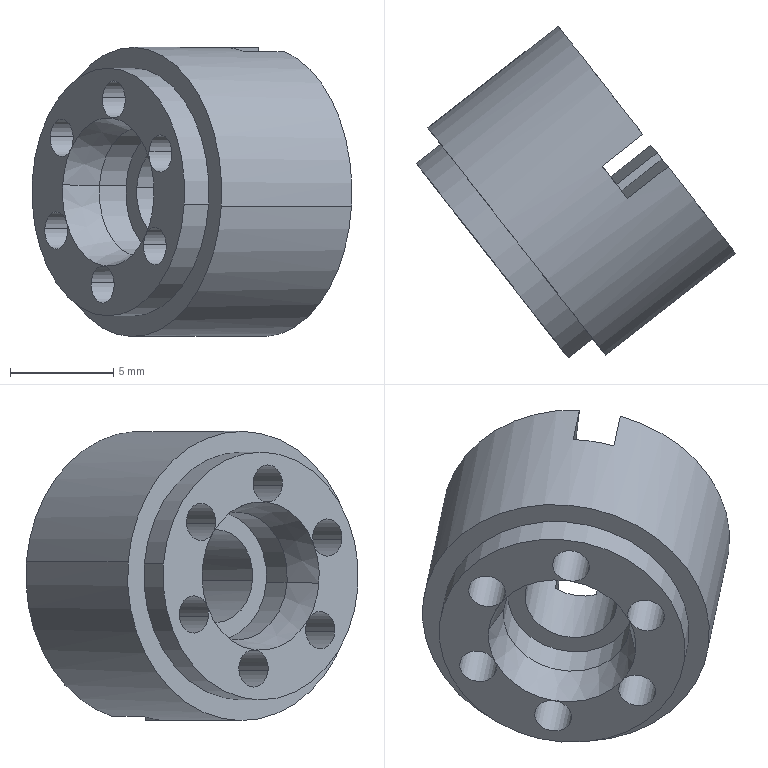Part | SolidWorks | features BaseBody 1 | 1 solid | 33 faces | box 15.49 x 16.093 x 14 mm | volume 1010 mm3 | cylinder 20 | plane 11 | cone 2 | commonest cylinder face diameters 1.8 x12 4.5 x2 6.2 x2 12 x2 14 x2
STEP:
#1=CARTESIAN_POINT('',(2.546,87.739,-118.333));
#2=VERTEX_POINT('',#1);
#3=CARTESIAN_POINT('',(-4.807,97.151,-117.167));
#4=VERTEX_POINT('',#3);
#5=CARTESIAN_POINT('',(-1.131,92.445,-117.75));
#6=DIRECTION('',(-0.788,-0.6157,0.));
#7=DIRECTION('',(0.6128,-0.7843,-0.09712));
#8=AXIS2_PLACEMENT_3D('',#5,#6,#7);
#9=CIRCLE('',#8,6.);
#10=EDGE_CURVE('',#2,#4,#9,.T.);
#11=ORIENTED_EDGE('',*,*,#10,.T.);
#12=CARTESIAN_POINT('',(-5.989,96.227,-117.167));
#13=VERTEX_POINT('',#12);
#14=CARTESIAN_POINT('',(-5.989,96.227,-117.167));
#15=DIRECTION('',(-0.788,-0.6157,0.));
#16=VECTOR('',#15,1000.);
#17=LINE('',#14,#16);
#18=EDGE_CURVE('',#4,#13,#17,.T.);
#19=ORIENTED_EDGE('',*,*,#18,.T.);
#20=CARTESIAN_POINT('',(1.364,86.816,-118.333));
#21=VERTEX_POINT('',#20);
#22=CARTESIAN_POINT('',(-2.313,91.521,-117.75));
#23=DIRECTION('',(-0.788,-0.6157,0.));
#24=DIRECTION('',(0.6128,-0.7843,-0.09712));
#25=AXIS2_PLACEMENT_3D('',#22,#23,#24);
#26=CIRCLE('',#25,6.);
#27=EDGE_CURVE('',#21,#13,#26,.T.);
#28=ORIENTED_EDGE('',*,*,#27,.F.);
#29=CARTESIAN_POINT('',(1.364,86.816,-118.333));
#30=DIRECTION('',(-0.788,-0.6157,0.));
#31=VECTOR('',#30,1000.);
#32=LINE('',#29,#31);
#33=EDGE_CURVE('',#2,#21,#32,.T.);
#34=ORIENTED_EDGE('',*,*,#33,.F.);
#35=EDGE_LOOP('',(#11,#19,#28,#34));
#36=FACE_OUTER_BOUND('',#35,.T.);
#37=CARTESIAN_POINT('',(-2.313,91.521,-117.75));
#38=DIRECTION('',(-0.788,-0.6157,0.));
#39=DIRECTION('',(0.6128,-0.7843,-0.09712));
#40=AXIS2_PLACEMENT_3D('',#37,#38,#39);
#41=CYLINDRICAL_SURFACE('',#40,6.);
#42=ADVANCED_FACE('',(#36),#41,.T.);
#43=CARTESIAN_POINT('',(-2.742,95.102,-117.449));
#44=VERTEX_POINT('',#43);
#45=CARTESIAN_POINT('',(1.057,90.239,-118.051));
#46=VERTEX_POINT('',#45);
#47=CARTESIAN_POINT('',(-0.8423,92.67,-117.75));
#48=DIRECTION('',(-0.788,-0.6157,0.));
#49=DIRECTION('',(0.6128,-0.7843,-0.09712));
#50=AXIS2_PLACEMENT_3D('',#47,#48,#49);
#51=CIRCLE('',#50,3.1);
#52=EDGE_CURVE('',#44,#46,#51,.T.);
#53=ORIENTED_EDGE('',*,*,#52,.F.);
#54=CARTESIAN_POINT('',(-4.519,94.345,-117.4));
#55=VERTEX_POINT('',#54);
#56=CARTESIAN_POINT('',(-2.742,95.102,-117.449));
#57=DIRECTION('',(-0.9198,-0.3917,0.02514));
#58=VECTOR('',#57,1000.);
#59=LINE('',#56,#58);
#60=EDGE_CURVE('',#44,#55,#59,.T.);
#61=ORIENTED_EDGE('',*,*,#60,.T.);
#62=CARTESIAN_POINT('',(-4.331,94.104,-119.239));
#63=VERTEX_POINT('',#62);
#64=CARTESIAN_POINT('',(-2.313,91.521,-117.75));
#65=DIRECTION('',(-0.788,-0.6157,0.));
#66=DIRECTION('',(0.6128,-0.7843,-0.09712));
#67=AXIS2_PLACEMENT_3D('',#64,#65,#66);
#68=CIRCLE('',#67,3.6);
#69=EDGE_CURVE('',#55,#63,#68,.T.);
#70=ORIENTED_EDGE('',*,*,#69,.T.);
#71=CARTESIAN_POINT('',(-2.528,91.797,-121.333));
#72=VERTEX_POINT('',#71);
#73=CARTESIAN_POINT('',(-2.313,91.521,-117.75));
#74=DIRECTION('',(-0.788,-0.6157,0.));
#75=DIRECTION('',(0.6128,-0.7843,-0.09712));
#76=AXIS2_PLACEMENT_3D('',#73,#74,#75);
#77=CIRCLE('',#76,3.6);
#78=EDGE_CURVE('',#63,#72,#77,.T.);
#79=ORIENTED_EDGE('',*,*,#78,.T.);
#80=CARTESIAN_POINT('',(-0.51,89.214,-119.844));
#81=VERTEX_POINT('',#80);
#82=CARTESIAN_POINT('',(-2.313,91.521,-117.75));
#83=DIRECTION('',(-0.788,-0.6157,0.));
#84=DIRECTION('',(0.6128,-0.7843,-0.09712));
#85=AXIS2_PLACEMENT_3D('',#82,#83,#84);
#86=CIRCLE('',#85,3.6);
#87=EDGE_CURVE('',#72,#81,#86,.T.);
#88=ORIENTED_EDGE('',*,*,#87,.T.);
#89=CARTESIAN_POINT('',(-0.1068,88.698,-118.1));
#90=VERTEX_POINT('',#89);
#91=CARTESIAN_POINT('',(-2.313,91.521,-117.75));
#92=DIRECTION('',(-0.788,-0.6157,0.));
#93=DIRECTION('',(0.6128,-0.7843,-0.09712));
#94=AXIS2_PLACEMENT_3D('',#91,#92,#93);
#95=CIRCLE('',#94,3.6);
#96=EDGE_CURVE('',#81,#90,#95,.T.);
#97=ORIENTED_EDGE('',*,*,#96,.T.);
#98=CARTESIAN_POINT('',(1.057,90.239,-118.051));
#99=DIRECTION('',(-0.6026,-0.7977,-0.02514));
#100=VECTOR('',#99,1000.);
#101=LINE('',#98,#100);
#102=EDGE_CURVE('',#46,#90,#101,.T.);
#103=ORIENTED_EDGE('',*,*,#102,.F.);
#104=EDGE_LOOP('',(#53,#61,#70,#79,#88,#97,#103));
#105=FACE_OUTER_BOUND('',#104,.T.);
#106=CARTESIAN_POINT('',(-0.8423,92.67,-117.75));
#107=DIRECTION('',(-0.788,-0.6157,0.));
#108=DIRECTION('',(0.6128,-0.7843,-0.09712));
#109=AXIS2_PLACEMENT_3D('',#106,#107,#108);
#110=CONICAL_SURFACE('',#109,3.1,0.2618);
#111=ADVANCED_FACE('',(#105),#110,.F.);
#112=CARTESIAN_POINT('',(-1.454,96.108,-117.449));
#113=VERTEX_POINT('',#112);
#114=CARTESIAN_POINT('',(2.345,91.245,-118.051));
#115=VERTEX_POINT('',#114);
#116=CARTESIAN_POINT('',(0.4453,93.676,-117.75));
#117=DIRECTION('',(-0.788,-0.6157,0.));
#118=DIRECTION('',(0.6128,-0.7843,-0.09712));
#119=AXIS2_PLACEMENT_3D('',#116,#117,#118);
#120=CIRCLE('',#119,3.1);
#121=EDGE_CURVE('',#113,#115,#120,.T.);
#122=ORIENTED_EDGE('',*,*,#121,.F.);
#123=CARTESIAN_POINT('',(-4.212,93.953,-117.449));
#124=DIRECTION('',(-0.788,-0.6157,0.));
#125=VECTOR('',#124,1000.);
#126=LINE('',#123,#125);
#127=EDGE_CURVE('',#113,#44,#126,.T.);
#128=ORIENTED_EDGE('',*,*,#127,.T.);
#129=ORIENTED_EDGE('',*,*,#52,.T.);
#130=CARTESIAN_POINT('',(-0.4132,89.09,-118.051));
#131=DIRECTION('',(-0.788,-0.6157,0.));
#132=VECTOR('',#131,1000.);
#133=LINE('',#130,#132);
#134=EDGE_CURVE('',#115,#46,#133,.T.);
#135=ORIENTED_EDGE('',*,*,#134,.F.);
#136=EDGE_LOOP('',(#122,#128,#129,#135));
#137=FACE_OUTER_BOUND('',#136,.T.);
#138=CARTESIAN_POINT('',(-2.313,91.521,-117.75));
#139=DIRECTION('',(-0.788,-0.6157,0.));
#140=DIRECTION('',(0.6128,-0.7843,-0.09712));
#141=AXIS2_PLACEMENT_3D('',#138,#139,#140);
#142=CYLINDRICAL_SURFACE('',#141,3.1);
#143=ADVANCED_FACE('',(#137),#142,.F.);
#144=CARTESIAN_POINT('',(3.795,99.135,-117.531));
#145=VERTEX_POINT('',#144);
#146=CARTESIAN_POINT('',(4.44,98.309,-119.659));
#147=VERTEX_POINT('',#146);
#148=CARTESIAN_POINT('',(5.173,97.37,-117.75));
#149=DIRECTION('',(-0.788,-0.6157,0.));
#150=DIRECTION('',(0.6128,-0.7843,-0.09712));
#151=AXIS2_PLACEMENT_3D('',#148,#149,#150);
#152=CIRCLE('',#151,2.25);
#153=EDGE_CURVE('',#145,#147,#152,.T.);
#154=ORIENTED_EDGE('',*,*,#153,.F.);
#155=CARTESIAN_POINT('',(-0.9334,95.441,-117.531));
#156=VERTEX_POINT('',#155);
#157=CARTESIAN_POINT('',(-3.691,93.286,-117.531));
#158=DIRECTION('',(-0.788,-0.6157,0.));
#159=VECTOR('',#158,1000.);
#160=LINE('',#157,#159);
#161=EDGE_CURVE('',#145,#156,#160,.T.);
#162=ORIENTED_EDGE('',*,*,#161,.T.);
#163=CARTESIAN_POINT('',(1.824,91.912,-117.969));
#164=VERTEX_POINT('',#163);
#165=CARTESIAN_POINT('',(0.4453,93.676,-117.75));
#166=DIRECTION('',(-0.788,-0.6157,0.));
#167=DIRECTION('',(0.6128,-0.7843,-0.09712));
#168=AXIS2_PLACEMENT_3D('',#165,#166,#167);
#169=CIRCLE('',#168,2.25);
#170=EDGE_CURVE('',#156,#164,#169,.T.);
#171=ORIENTED_EDGE('',*,*,#170,.T.);
#172=CARTESIAN_POINT('',(6.552,95.606,-117.969));
#173=VERTEX_POINT('',#172);
#174=CARTESIAN_POINT('',(-0.934,89.757,-117.969));
#175=DIRECTION('',(-0.788,-0.6157,0.));
#176=VECTOR('',#175,1000.);
#177=LINE('',#174,#176);
#178=EDGE_CURVE('',#173,#164,#177,.T.);
#179=ORIENTED_EDGE('',*,*,#178,.F.);
#180=CARTESIAN_POINT('',(5.666,96.74,-119.853));
#181=VERTEX_POINT('',#180);
#182=CARTESIAN_POINT('',(5.173,97.37,-117.75));
#183=DIRECTION('',(-0.788,-0.6157,0.));
#184=DIRECTION('',(0.6128,-0.7843,-0.09712));
#185=AXIS2_PLACEMENT_3D('',#182,#183,#184);
#186=CIRCLE('',#185,2.25);
#187=EDGE_CURVE('',#181,#173,#186,.T.);
#188=ORIENTED_EDGE('',*,*,#187,.F.);
#189=CARTESIAN_POINT('',(3.696,95.201,-119.853));
#190=VERTEX_POINT('',#189);
#191=CARTESIAN_POINT('',(-1.82,90.891,-119.853));
#192=DIRECTION('',(0.788,0.6157,0.));
#193=VECTOR('',#192,1000.);
#194=LINE('',#191,#193);
#195=EDGE_CURVE('',#190,#181,#194,.T.);
#196=ORIENTED_EDGE('',*,*,#195,.F.);
#197=CARTESIAN_POINT('',(2.47,96.77,-119.659));
#198=VERTEX_POINT('',#197);
#199=CARTESIAN_POINT('',(3.203,95.831,-117.75));
#200=DIRECTION('',(0.788,0.6157,0.));
#201=DIRECTION('',(-0.6128,0.7843,0.09712));
#202=AXIS2_PLACEMENT_3D('',#199,#200,#201);
#203=CIRCLE('',#202,2.25);
#204=EDGE_CURVE('',#190,#198,#203,.T.);
#205=ORIENTED_EDGE('',*,*,#204,.T.);
#206=CARTESIAN_POINT('',(-3.046,92.46,-119.659));
#207=DIRECTION('',(-0.788,-0.6157,0.));
#208=VECTOR('',#207,1000.);
#209=LINE('',#206,#208);
#210=EDGE_CURVE('',#147,#198,#209,.T.);
#211=ORIENTED_EDGE('',*,*,#210,.F.);
#212=EDGE_LOOP('',(#154,#162,#171,#179,#188,#196,#205,#211));
#213=FACE_OUTER_BOUND('',#212,.T.);
#214=CARTESIAN_POINT('',(-2.313,91.521,-117.75));
#215=DIRECTION('',(-0.788,-0.6157,0.));
#216=DIRECTION('',(0.6128,-0.7843,-0.09712));
#217=AXIS2_PLACEMENT_3D('',#214,#215,#216);
#218=CYLINDRICAL_SURFACE('',#217,2.25);
#219=ADVANCED_FACE('',(#213),#218,.F.);
#220=CARTESIAN_POINT('',(4.975,97.624,-110.757));
#221=VERTEX_POINT('',#220);
#222=CARTESIAN_POINT('',(0.8841,102.86,-117.07));
#223=VERTEX_POINT('',#222);
#224=CARTESIAN_POINT('',(5.173,97.37,-117.75));
#225=DIRECTION('',(-0.788,-0.6157,0.));
#226=DIRECTION('',(0.6128,-0.7843,-0.09712));
#227=AXIS2_PLACEMENT_3D('',#224,#225,#226);
#228=CIRCLE('',#227,7.);
#229=EDGE_CURVE('',#221,#223,#228,.T.);
#230=ORIENTED_EDGE('',*,*,#229,.T.);
#231=CARTESIAN_POINT('',(-5.42,97.935,-117.07));
#232=VERTEX_POINT('',#231);
#233=CARTESIAN_POINT('',(-6.602,97.011,-117.07));
#234=DIRECTION('',(-0.788,-0.6157,0.));
#235=VECTOR('',#234,1000.);
#236=LINE('',#233,#235);
#237=EDGE_CURVE('',#223,#232,#236,.T.);
#238=ORIENTED_EDGE('',*,*,#237,.T.);
#239=CARTESIAN_POINT('',(3.159,86.955,-118.43));
#240=VERTEX_POINT('',#239);
#241=CARTESIAN_POINT('',(-1.131,92.445,-117.75));
#242=DIRECTION('',(-0.788,-0.6157,0.));
#243=DIRECTION('',(0.6128,-0.7843,-0.09712));
#244=AXIS2_PLACEMENT_3D('',#241,#242,#243);
#245=CIRCLE('',#244,7.);
#246=EDGE_CURVE('',#240,#232,#245,.T.);
#247=ORIENTED_EDGE('',*,*,#246,.F.);
#248=CARTESIAN_POINT('',(9.463,91.88,-118.43));
#249=VERTEX_POINT('',#248);
#250=CARTESIAN_POINT('',(1.977,86.031,-118.43));
#251=DIRECTION('',(-0.788,-0.6157,0.));
#252=VECTOR('',#251,1000.);
#253=LINE('',#250,#252);
#254=EDGE_CURVE('',#249,#240,#253,.T.);
#255=ORIENTED_EDGE('',*,*,#254,.F.);
#256=CARTESIAN_POINT('',(6.2,96.056,-110.952));
#257=VERTEX_POINT('',#256);
#258=CARTESIAN_POINT('',(5.173,97.37,-117.75));
#259=DIRECTION('',(-0.788,-0.6157,0.));
#260=DIRECTION('',(0.6128,-0.7843,-0.09712));
#261=AXIS2_PLACEMENT_3D('',#258,#259,#260);
#262=CIRCLE('',#261,7.);
#263=EDGE_CURVE('',#249,#257,#262,.T.);
#264=ORIENTED_EDGE('',*,*,#263,.T.);
#265=CARTESIAN_POINT('',(4.23,94.517,-110.952));
#266=VERTEX_POINT('',#265);
#267=CARTESIAN_POINT('',(4.23,94.517,-110.952));
#268=DIRECTION('',(0.788,0.6157,0.));
#269=VECTOR('',#268,1000.);
#270=LINE('',#267,#269);
#271=EDGE_CURVE('',#266,#257,#270,.T.);
#272=ORIENTED_EDGE('',*,*,#271,.F.);
#273=CARTESIAN_POINT('',(3.005,96.085,-110.757));
#274=VERTEX_POINT('',#273);
#275=CARTESIAN_POINT('',(3.203,95.831,-117.75));
#276=DIRECTION('',(0.788,0.6157,0.));
#277=DIRECTION('',(-0.6128,0.7843,0.09712));
#278=AXIS2_PLACEMENT_3D('',#275,#276,#277);
#279=CIRCLE('',#278,7.);
#280=EDGE_CURVE('',#274,#266,#279,.T.);
#281=ORIENTED_EDGE('',*,*,#280,.F.);
#282=CARTESIAN_POINT('',(3.005,96.085,-110.757));
#283=DIRECTION('',(0.788,0.6157,0.));
#284=VECTOR('',#283,1000.);
#285=LINE('',#282,#284);
#286=EDGE_CURVE('',#274,#221,#285,.T.);
#287=ORIENTED_EDGE('',*,*,#286,.T.);
#288=EDGE_LOOP('',(#230,#238,#247,#255,#264,#272,#281,#287));
#289=FACE_OUTER_BOUND('',#288,.T.);
#290=CARTESIAN_POINT('',(-2.313,91.521,-117.75));
#291=DIRECTION('',(-0.788,-0.6157,0.));
#292=DIRECTION('',(0.6128,-0.7843,-0.09712));
#293=AXIS2_PLACEMENT_3D('',#290,#291,#292);
#294=CYLINDRICAL_SURFACE('',#293,7.);
#295=ADVANCED_FACE('',(#289),#294,.T.);
#296=CARTESIAN_POINT('',(-1.492,90.471,-113.359));
#297=VERTEX_POINT('',#296);
#298=CARTESIAN_POINT('',(-2.097,91.246,-114.167));
#299=VERTEX_POINT('',#298);
#300=CARTESIAN_POINT('',(-2.044,91.177,-113.271));
#301=DIRECTION('',(0.788,0.6157,0.));
#302=DIRECTION('',(-0.6128,0.7843,0.09712));
#303=AXIS2_PLACEMENT_3D('',#300,#301,#302);
#304=CIRCLE('',#303,0.9);
#305=EDGE_CURVE('',#297,#299,#304,.T.);
#306=ORIENTED_EDGE('',*,*,#305,.F.);
#307=CARTESIAN_POINT('',(4.024,94.781,-113.359));
#308=VERTEX_POINT('',#307);
#309=CARTESIAN_POINT('',(-1.492,90.471,-113.359));
#310=DIRECTION('',(0.788,0.6157,0.));
#311=VECTOR('',#310,1000.);
#312=LINE('',#309,#311);
#313=EDGE_CURVE('',#297,#308,#312,.T.);
#314=ORIENTED_EDGE('',*,*,#313,.T.);
#315=CARTESIAN_POINT('',(2.921,96.192,-113.184));
#316=VERTEX_POINT('',#315);
#317=CARTESIAN_POINT('',(3.472,95.487,-113.271));
#318=DIRECTION('',(0.788,0.6157,0.));
#319=DIRECTION('',(-0.6128,0.7843,0.09712));
#320=AXIS2_PLACEMENT_3D('',#317,#318,#319);
#321=CIRCLE('',#320,0.9);
#322=EDGE_CURVE('',#308,#316,#321,.T.);
#323=ORIENTED_EDGE('',*,*,#322,.T.);
#324=CARTESIAN_POINT('',(-2.595,91.883,-113.184));
#325=VERTEX_POINT('',#324);
#326=CARTESIAN_POINT('',(-2.595,91.883,-113.184));
#327=DIRECTION('',(0.788,0.6157,0.));
#328=VECTOR('',#327,1000.);
#329=LINE('',#326,#328);
#330=EDGE_CURVE('',#325,#316,#329,.T.);
#331=ORIENTED_EDGE('',*,*,#330,.F.);
#332=CARTESIAN_POINT('',(-2.044,91.177,-113.271));
#333=DIRECTION('',(0.788,0.6157,0.));
#334=DIRECTION('',(-0.6128,0.7843,0.09712));
#335=AXIS2_PLACEMENT_3D('',#332,#333,#334);
#336=CIRCLE('',#335,0.9);
#337=EDGE_CURVE('',#299,#325,#336,.T.);
#338=ORIENTED_EDGE('',*,*,#337,.F.);
#339=EDGE_LOOP('',(#306,#314,#323,#331,#338));
#340=FACE_OUTER_BOUND('',#339,.T.);
#341=CARTESIAN_POINT('',(-2.044,91.177,-113.271));
#342=DIRECTION('',(0.788,0.6157,0.));
#343=DIRECTION('',(-0.6128,0.7843,0.09712));
#344=AXIS2_PLACEMENT_3D('',#341,#342,#343);
#345=CYLINDRICAL_SURFACE('',#344,0.9);
#346=ADVANCED_FACE('',(#340),#345,.F.);
#347=CARTESIAN_POINT('',(-4.015,93.7,-115.22));
#348=VERTEX_POINT('',#347);
#349=CARTESIAN_POINT('',(-4.115,93.829,-115.656));
#350=VERTEX_POINT('',#349);
#351=CARTESIAN_POINT('',(-4.566,94.406,-115.132));
#352=DIRECTION('',(0.788,0.6157,0.));
#353=DIRECTION('',(-0.6128,0.7843,0.09712));
#354=AXIS2_PLACEMENT_3D('',#351,#352,#353);
#355=CIRCLE('',#354,0.9);
#356=EDGE_CURVE('',#348,#350,#355,.T.);
#357=ORIENTED_EDGE('',*,*,#356,.F.);
#358=CARTESIAN_POINT('',(3.471,99.549,-115.22));
#359=VERTEX_POINT('',#358);
#360=CARTESIAN_POINT('',(-4.015,93.7,-115.22));
#361=DIRECTION('',(0.788,0.6157,0.));
#362=VECTOR('',#361,1000.);
#363=LINE('',#360,#362);
#364=EDGE_CURVE('',#348,#359,#363,.T.);
#365=ORIENTED_EDGE('',*,*,#364,.T.);
#366=CARTESIAN_POINT('',(2.368,100.96,-115.045));
#367=VERTEX_POINT('',#366);
#368=CARTESIAN_POINT('',(2.92,100.254,-115.132));
#369=DIRECTION('',(0.788,0.6157,0.));
#370=DIRECTION('',(-0.6128,0.7843,0.09712));
#371=AXIS2_PLACEMENT_3D('',#368,#369,#370);
#372=CIRCLE('',#371,0.9);
#373=EDGE_CURVE('',#359,#367,#372,.T.);
#374=ORIENTED_EDGE('',*,*,#373,.T.);
#375=CARTESIAN_POINT('',(-5.118,95.112,-115.045));
#376=VERTEX_POINT('',#375);
#377=CARTESIAN_POINT('',(-5.118,95.112,-115.045));
#378=DIRECTION('',(0.788,0.6157,0.));
#379=VECTOR('',#378,1000.);
#380=LINE('',#377,#379);
#381=EDGE_CURVE('',#376,#367,#380,.T.);
#382=ORIENTED_EDGE('',*,*,#381,.F.);
#383=CARTESIAN_POINT('',(-4.566,94.406,-115.132));
#384=DIRECTION('',(0.788,0.6157,0.));
#385=DIRECTION('',(-0.6128,0.7843,0.09712));
#386=AXIS2_PLACEMENT_3D('',#383,#384,#385);
#387=CIRCLE('',#386,0.9);
#388=EDGE_CURVE('',#350,#376,#387,.T.);
#389=ORIENTED_EDGE('',*,*,#388,.F.);
#390=EDGE_LOOP('',(#357,#365,#374,#382,#389));
#391=FACE_OUTER_BOUND('',#390,.T.);
#392=CARTESIAN_POINT('',(-4.566,94.406,-115.132));
#393=DIRECTION('',(0.788,0.6157,0.));
#394=DIRECTION('',(-0.6128,0.7843,0.09712));
#395=AXIS2_PLACEMENT_3D('',#392,#393,#394);
#396=CYLINDRICAL_SURFACE('',#395,0.9);
#397=ADVANCED_FACE('',(#391),#396,.F.);
#398=CARTESIAN_POINT('',(-4.284,94.044,-119.698));
#399=VERTEX_POINT('',#398);
#400=CARTESIAN_POINT('',(-5.387,95.456,-119.523));
#401=VERTEX_POINT('',#400);
#402=CARTESIAN_POINT('',(-4.835,94.75,-119.611));
#403=DIRECTION('',(0.788,0.6157,0.));
#404=DIRECTION('',(-0.6128,0.7843,0.09712));
#405=AXIS2_PLACEMENT_3D('',#402,#403,#404);
#406=CIRCLE('',#405,0.9);
#407=EDGE_CURVE('',#399,#401,#406,.T.);
#408=ORIENTED_EDGE('',*,*,#407,.F.);
#409=CARTESIAN_POINT('',(3.202,99.893,-119.698));
#410=VERTEX_POINT('',#409);
#411=CARTESIAN_POINT('',(-4.284,94.044,-119.698));
#412=DIRECTION('',(0.788,0.6157,0.));
#413=VECTOR('',#412,1000.);
#414=LINE('',#411,#413);
#415=EDGE_CURVE('',#399,#410,#414,.T.);
#416=ORIENTED_EDGE('',*,*,#415,.T.);
#417=CARTESIAN_POINT('',(2.099,101.305,-119.523));
#418=VERTEX_POINT('',#417);
#419=CARTESIAN_POINT('',(2.651,100.599,-119.611));
#420=DIRECTION('',(0.788,0.6157,0.));
#421=DIRECTION('',(-0.6128,0.7843,0.09712));
#422=AXIS2_PLACEMENT_3D('',#419,#420,#421);
#423=CIRCLE('',#422,0.9);
#424=EDGE_CURVE('',#410,#418,#423,.T.);
#425=ORIENTED_EDGE('',*,*,#424,.T.);
#426=CARTESIAN_POINT('',(-5.387,95.456,-119.523));
#427=DIRECTION('',(0.788,0.6157,0.));
#428=VECTOR('',#427,1000.);
#429=LINE('',#426,#428);
#430=EDGE_CURVE('',#401,#418,#429,.T.);
#431=ORIENTED_EDGE('',*,*,#430,.F.);
#432=EDGE_LOOP('',(#408,#416,#425,#431));
#433=FACE_OUTER_BOUND('',#432,.T.);
#434=CARTESIAN_POINT('',(-4.835,94.75,-119.611));
#435=DIRECTION('',(0.788,0.6157,0.));
#436=DIRECTION('',(-0.6128,0.7843,0.09712));
#437=AXIS2_PLACEMENT_3D('',#434,#435,#436);
#438=CYLINDRICAL_SURFACE('',#437,0.9);
#439=ADVANCED_FACE('',(#433),#438,.F.);
#440=CARTESIAN_POINT('',(-2.03,91.16,-122.316));
#441=VERTEX_POINT('',#440);
#442=CARTESIAN_POINT('',(-3.133,92.572,-122.141));
#443=VERTEX_POINT('',#442);
#444=CARTESIAN_POINT('',(-2.582,91.866,-122.229));
#445=DIRECTION('',(0.788,0.6157,0.));
#446=DIRECTION('',(-0.6128,0.7843,0.09712));
#447=AXIS2_PLACEMENT_3D('',#444,#445,#446);
#448=CIRCLE('',#447,0.9);
#449=EDGE_CURVE('',#441,#443,#448,.T.);
#450=ORIENTED_EDGE('',*,*,#449,.F.);
#451=CARTESIAN_POINT('',(3.486,95.47,-122.316));
#452=VERTEX_POINT('',#451);
#453=CARTESIAN_POINT('',(-2.03,91.16,-122.316));
#454=DIRECTION('',(0.788,0.6157,0.));
#455=VECTOR('',#454,1000.);
#456=LINE('',#453,#455);
#457=EDGE_CURVE('',#441,#452,#456,.T.);
#458=ORIENTED_EDGE('',*,*,#457,.T.);
#459=CARTESIAN_POINT('',(2.383,96.881,-122.141));
#460=VERTEX_POINT('',#459);
#461=CARTESIAN_POINT('',(2.934,96.175,-122.229));
#462=DIRECTION('',(0.788,0.6157,0.));
#463=DIRECTION('',(-0.6128,0.7843,0.09712));
#464=AXIS2_PLACEMENT_3D('',#461,#462,#463);
#465=CIRCLE('',#464,0.9);
#466=EDGE_CURVE('',#452,#460,#465,.T.);
#467=ORIENTED_EDGE('',*,*,#466,.T.);
#468=CARTESIAN_POINT('',(-3.133,92.572,-122.141));
#469=DIRECTION('',(0.788,0.6157,0.));
#470=VECTOR('',#469,1000.);
#471=LINE('',#468,#470);
#472=EDGE_CURVE('',#443,#460,#471,.T.);
#473=ORIENTED_EDGE('',*,*,#472,.F.);
#474=EDGE_LOOP('',(#450,#458,#467,#473));
#475=FACE_OUTER_BOUND('',#474,.T.);
#476=CARTESIAN_POINT('',(-2.582,91.866,-122.229));
#477=DIRECTION('',(0.788,0.6157,0.));
#478=DIRECTION('',(-0.6128,0.7843,0.09712));
#479=AXIS2_PLACEMENT_3D('',#476,#477,#478);
#480=CYLINDRICAL_SURFACE('',#479,0.9);
#481=ADVANCED_FACE('',(#475),#480,.F.);
#482=CARTESIAN_POINT('',(0.4922,87.931,-120.455));
#483=VERTEX_POINT('',#482);
#484=CARTESIAN_POINT('',(-0.6108,89.343,-120.28));
#485=VERTEX_POINT('',#484);
#486=CARTESIAN_POINT('',(-0.05931,88.637,-120.368));
#487=DIRECTION('',(0.788,0.6157,0.));
#488=DIRECTION('',(-0.6128,0.7843,0.09712));
#489=AXIS2_PLACEMENT_3D('',#486,#487,#488);
#490=CIRCLE('',#489,0.9);
#491=EDGE_CURVE('',#483,#485,#490,.T.);
#492=ORIENTED_EDGE('',*,*,#491,.F.);
#493=CARTESIAN_POINT('',(7.978,93.78,-120.455));
#494=VERTEX_POINT('',#493);
#495=CARTESIAN_POINT('',(0.4922,87.931,-120.455));
#496=DIRECTION('',(0.788,0.6157,0.));
#497=VECTOR('',#496,1000.);
#498=LINE('',#495,#497);
#499=EDGE_CURVE('',#483,#494,#498,.T.);
#500=ORIENTED_EDGE('',*,*,#499,.T.);
#501=CARTESIAN_POINT('',(6.875,95.192,-120.28));
#502=VERTEX_POINT('',#501);
#503=CARTESIAN_POINT('',(7.427,94.486,-120.368));
#504=DIRECTION('',(0.788,0.6157,0.));
#505=DIRECTION('',(-0.6128,0.7843,0.09712));
#506=AXIS2_PLACEMENT_3D('',#503,#504,#505);
#507=CIRCLE('',#506,0.9);
#508=EDGE_CURVE('',#494,#502,#507,.T.);
#509=ORIENTED_EDGE('',*,*,#508,.T.);
#510=CARTESIAN_POINT('',(-0.6108,89.343,-120.28));
#511=DIRECTION('',(0.788,0.6157,0.));
#512=VECTOR('',#511,1000.);
#513=LINE('',#510,#512);
#514=EDGE_CURVE('',#485,#502,#513,.T.);
#515=ORIENTED_EDGE('',*,*,#514,.F.);
#516=EDGE_LOOP('',(#492,#500,#509,#515));
#517=FACE_OUTER_BOUND('',#516,.T.);
#518=CARTESIAN_POINT('',(-0.05931,88.637,-120.368));
#519=DIRECTION('',(0.788,0.6157,0.));
#520=DIRECTION('',(-0.6128,0.7843,0.09712));
#521=AXIS2_PLACEMENT_3D('',#518,#519,#520);
#522=CYLINDRICAL_SURFACE('',#521,0.9);
#523=ADVANCED_FACE('',(#517),#522,.F.);
#524=CARTESIAN_POINT('',(0.7612,87.587,-115.977));
#525=VERTEX_POINT('',#524);
#526=CARTESIAN_POINT('',(-0.2947,88.938,-116.261));
#527=VERTEX_POINT('',#526);
#528=CARTESIAN_POINT('',(0.2098,88.293,-115.889));
#529=DIRECTION('',(0.788,0.6157,0.));
#530=DIRECTION('',(-0.6128,0.7843,0.09712));
#531=AXIS2_PLACEMENT_3D('',#528,#529,#530);
#532=CIRCLE('',#531,0.9);
#533=EDGE_CURVE('',#525,#527,#532,.T.);
#534=ORIENTED_EDGE('',*,*,#533,.F.);
#535=CARTESIAN_POINT('',(8.247,93.436,-115.977));
#536=VERTEX_POINT('',#535);
#537=CARTESIAN_POINT('',(0.7612,87.587,-115.977));
#538=DIRECTION('',(0.788,0.6157,0.));
#539=VECTOR('',#538,1000.);
#540=LINE('',#537,#539);
#541=EDGE_CURVE('',#525,#536,#540,.T.);
#542=ORIENTED_EDGE('',*,*,#541,.T.);
#543=CARTESIAN_POINT('',(7.144,94.847,-115.802));
#544=VERTEX_POINT('',#543);
#545=CARTESIAN_POINT('',(7.696,94.142,-115.889));
#546=DIRECTION('',(0.788,0.6157,0.));
#547=DIRECTION('',(-0.6128,0.7843,0.09712));
#548=AXIS2_PLACEMENT_3D('',#545,#546,#547);
#549=CIRCLE('',#548,0.9);
#550=EDGE_CURVE('',#536,#544,#549,.T.);
#551=ORIENTED_EDGE('',*,*,#550,.T.);
#552=CARTESIAN_POINT('',(-0.3417,88.999,-115.802));
#553=VERTEX_POINT('',#552);
#554=CARTESIAN_POINT('',(-0.3417,88.999,-115.802));
#555=DIRECTION('',(0.788,0.6157,0.));
#556=VECTOR('',#555,1000.);
#557=LINE('',#554,#556);
#558=EDGE_CURVE('',#553,#544,#557,.T.);
#559=ORIENTED_EDGE('',*,*,#558,.F.);
#560=CARTESIAN_POINT('',(0.2098,88.293,-115.889));
#561=DIRECTION('',(0.788,0.6157,0.));
#562=DIRECTION('',(-0.6128,0.7843,0.09712));
#563=AXIS2_PLACEMENT_3D('',#560,#561,#562);
#564=CIRCLE('',#563,0.9);
#565=EDGE_CURVE('',#527,#553,#564,.T.);
#566=ORIENTED_EDGE('',*,*,#565,.F.);
#567=EDGE_LOOP('',(#534,#542,#551,#559,#566));
#568=FACE_OUTER_BOUND('',#567,.T.);
#569=CARTESIAN_POINT('',(0.2098,88.293,-115.889));
#570=DIRECTION('',(0.788,0.6157,0.));
#571=DIRECTION('',(-0.6128,0.7843,0.09712));
#572=AXIS2_PLACEMENT_3D('',#569,#570,#571);
#573=CYLINDRICAL_SURFACE('',#572,0.9);
#574=ADVANCED_FACE('',(#568),#573,.F.);
#575=ORIENTED_EDGE('',*,*,#541,.F.);
#576=CARTESIAN_POINT('',(0.2098,88.293,-115.889));
#577=DIRECTION('',(0.788,0.6157,0.));
#578=DIRECTION('',(-0.6128,0.7843,0.09712));
#579=AXIS2_PLACEMENT_3D('',#576,#577,#578);
#580=CIRCLE('',#579,0.9);
#581=EDGE_CURVE('',#553,#525,#580,.T.);
#582=ORIENTED_EDGE('',*,*,#581,.F.);
#583=ORIENTED_EDGE('',*,*,#558,.T.);
#584=CARTESIAN_POINT('',(7.696,94.142,-115.889));
#585=DIRECTION('',(0.788,0.6157,0.));
#586=DIRECTION('',(-0.6128,0.7843,0.09712));
#587=AXIS2_PLACEMENT_3D('',#584,#585,#586);
#588=CIRCLE('',#587,0.9);
#589=EDGE_CURVE('',#544,#536,#588,.T.);
#590=ORIENTED_EDGE('',*,*,#589,.T.);
#591=EDGE_LOOP('',(#575,#582,#583,#590));
#592=FACE_OUTER_BOUND('',#591,.T.);
#593=CARTESIAN_POINT('',(0.2098,88.293,-115.889));
#594=DIRECTION('',(0.788,0.6157,0.));
#595=DIRECTION('',(-0.6128,0.7843,0.09712));
#596=AXIS2_PLACEMENT_3D('',#593,#594,#595);
#597=CYLINDRICAL_SURFACE('',#596,0.9);
#598=ADVANCED_FACE('',(#592),#597,.F.);
#599=ORIENTED_EDGE('',*,*,#499,.F.);
#600=CARTESIAN_POINT('',(-0.05931,88.637,-120.368));
#601=DIRECTION('',(0.788,0.6157,0.));
#602=DIRECTION('',(-0.6128,0.7843,0.09712));
#603=AXIS2_PLACEMENT_3D('',#600,#601,#602);
#604=CIRCLE('',#603,0.9);
#605=EDGE_CURVE('',#81,#483,#604,.T.);
#606=ORIENTED_EDGE('',*,*,#605,.F.);
#607=CARTESIAN_POINT('',(-0.05931,88.637,-120.368));
#608=DIRECTION('',(0.788,0.6157,0.));
#609=DIRECTION('',(-0.6128,0.7843,0.09712));
#610=AXIS2_PLACEMENT_3D('',#607,#608,#609);
#611=CIRCLE('',#610,0.9);
#612=EDGE_CURVE('',#485,#81,#611,.T.);
#613=ORIENTED_EDGE('',*,*,#612,.F.);
#614=ORIENTED_EDGE('',*,*,#514,.T.);
#615=CARTESIAN_POINT('',(7.427,94.486,-120.368));
#616=DIRECTION('',(0.788,0.6157,0.));
#617=DIRECTION('',(-0.6128,0.7843,0.09712));
#618=AXIS2_PLACEMENT_3D('',#615,#616,#617);
#619=CIRCLE('',#618,0.9);
#620=EDGE_CURVE('',#502,#494,#619,.T.);
#621=ORIENTED_EDGE('',*,*,#620,.T.);
#622=EDGE_LOOP('',(#599,#606,#613,#614,#621));
#623=FACE_OUTER_BOUND('',#622,.T.);
#624=CARTESIAN_POINT('',(-0.05931,88.637,-120.368));
#625=DIRECTION('',(0.788,0.6157,0.));
#626=DIRECTION('',(-0.6128,0.7843,0.09712));
#627=AXIS2_PLACEMENT_3D('',#624,#625,#626);
#628=CYLINDRICAL_SURFACE('',#627,0.9);
#629=ADVANCED_FACE('',(#623),#628,.F.);
#630=ORIENTED_EDGE('',*,*,#457,.F.);
#631=CARTESIAN_POINT('',(-2.582,91.866,-122.229));
#632=DIRECTION('',(0.788,0.6157,0.));
#633=DIRECTION('',(-0.6128,0.7843,0.09712));
#634=AXIS2_PLACEMENT_3D('',#631,#632,#633);
#635=CIRCLE('',#634,0.9);
#636=EDGE_CURVE('',#72,#441,#635,.T.);
#637=ORIENTED_EDGE('',*,*,#636,.F.);
#638=CARTESIAN_POINT('',(-2.582,91.866,-122.229));
#639=DIRECTION('',(0.788,0.6157,0.));
#640=DIRECTION('',(-0.6128,0.7843,0.09712));
#641=AXIS2_PLACEMENT_3D('',#638,#639,#640);
#642=CIRCLE('',#641,0.9);
#643=EDGE_CURVE('',#443,#72,#642,.T.);
#644=ORIENTED_EDGE('',*,*,#643,.F.);
#645=ORIENTED_EDGE('',*,*,#472,.T.);
#646=CARTESIAN_POINT('',(2.934,96.175,-122.229));
#647=DIRECTION('',(0.788,0.6157,0.));
#648=DIRECTION('',(-0.6128,0.7843,0.09712));
#649=AXIS2_PLACEMENT_3D('',#646,#647,#648);
#650=CIRCLE('',#649,0.9);
#651=EDGE_CURVE('',#460,#452,#650,.T.);
#652=ORIENTED_EDGE('',*,*,#651,.T.);
#653=EDGE_LOOP('',(#630,#637,#644,#645,#652));
#654=FACE_OUTER_BOUND('',#653,.T.);
#655=CARTESIAN_POINT('',(-2.582,91.866,-122.229));
#656=DIRECTION('',(0.788,0.6157,0.));
#657=DIRECTION('',(-0.6128,0.7843,0.09712));
#658=AXIS2_PLACEMENT_3D('',#655,#656,#657);
#659=CYLINDRICAL_SURFACE('',#658,0.9);
#660=ADVANCED_FACE('',(#654),#659,.F.);
#661=ORIENTED_EDGE('',*,*,#415,.F.);
#662=CARTESIAN_POINT('',(-4.835,94.75,-119.611));
#663=DIRECTION('',(0.788,0.6157,0.));
#664=DIRECTION('',(-0.6128,0.7843,0.09712));
#665=AXIS2_PLACEMENT_3D('',#662,#663,#664);
#666=CIRCLE('',#665,0.9);
#667=EDGE_CURVE('',#63,#399,#666,.T.);
#668=ORIENTED_EDGE('',*,*,#667,.F.);
#669=CARTESIAN_POINT('',(-4.835,94.75,-119.611));
#670=DIRECTION('',(0.788,0.6157,0.));
#671=DIRECTION('',(-0.6128,0.7843,0.09712));
#672=AXIS2_PLACEMENT_3D('',#669,#670,#671);
#673=CIRCLE('',#672,0.9);
#674=EDGE_CURVE('',#401,#63,#673,.T.);
#675=ORIENTED_EDGE('',*,*,#674,.F.);
#676=ORIENTED_EDGE('',*,*,#430,.T.);
#677=CARTESIAN_POINT('',(2.651,100.599,-119.611));
#678=DIRECTION('',(0.788,0.6157,0.));
#679=DIRECTION('',(-0.6128,0.7843,0.09712));
#680=AXIS2_PLACEMENT_3D('',#677,#678,#679);
#681=CIRCLE('',#680,0.9);
#682=EDGE_CURVE('',#418,#410,#681,.T.);
#683=ORIENTED_EDGE('',*,*,#682,.T.);
#684=EDGE_LOOP('',(#661,#668,#675,#676,#683));
#685=FACE_OUTER_BOUND('',#684,.T.);
#686=CARTESIAN_POINT('',(-4.835,94.75,-119.611));
#687=DIRECTION('',(0.788,0.6157,0.));
#688=DIRECTION('',(-0.6128,0.7843,0.09712));
#689=AXIS2_PLACEMENT_3D('',#686,#687,#688);
#690=CYLINDRICAL_SURFACE('',#689,0.9);
#691=ADVANCED_FACE('',(#685),#690,.F.);
#692=ORIENTED_EDGE('',*,*,#364,.F.);
#693=CARTESIAN_POINT('',(-4.566,94.406,-115.132));
#694=DIRECTION('',(0.788,0.6157,0.));
#695=DIRECTION('',(-0.6128,0.7843,0.09712));
#696=AXIS2_PLACEMENT_3D('',#693,#694,#695);
#697=CIRCLE('',#696,0.9);
#698=EDGE_CURVE('',#376,#348,#697,.T.);
#699=ORIENTED_EDGE('',*,*,#698,.F.);
#700=ORIENTED_EDGE('',*,*,#381,.T.);
#701=CARTESIAN_POINT('',(2.92,100.254,-115.132));
#702=DIRECTION('',(0.788,0.6157,0.));
#703=DIRECTION('',(-0.6128,0.7843,0.09712));
#704=AXIS2_PLACEMENT_3D('',#701,#702,#703);
#705=CIRCLE('',#704,0.9);
#706=EDGE_CURVE('',#367,#359,#705,.T.);
#707=ORIENTED_EDGE('',*,*,#706,.T.);
#708=EDGE_LOOP('',(#692,#699,#700,#707));
#709=FACE_OUTER_BOUND('',#708,.T.);
#710=CARTESIAN_POINT('',(-4.566,94.406,-115.132));
#711=DIRECTION('',(0.788,0.6157,0.));
#712=DIRECTION('',(-0.6128,0.7843,0.09712));
#713=AXIS2_PLACEMENT_3D('',#710,#711,#712);
#714=CYLINDRICAL_SURFACE('',#713,0.9);
#715=ADVANCED_FACE('',(#709),#714,.F.);
#716=ORIENTED_EDGE('',*,*,#313,.F.);
#717=CARTESIAN_POINT('',(-2.044,91.177,-113.271));
#718=DIRECTION('',(0.788,0.6157,0.));
#719=DIRECTION('',(-0.6128,0.7843,0.09712));
#720=AXIS2_PLACEMENT_3D('',#717,#718,#719);
#721=CIRCLE('',#720,0.9);
#722=EDGE_CURVE('',#325,#297,#721,.T.);
#723=ORIENTED_EDGE('',*,*,#722,.F.);
#724=ORIENTED_EDGE('',*,*,#330,.T.);
#725=CARTESIAN_POINT('',(3.472,95.487,-113.271));
#726=DIRECTION('',(0.788,0.6157,0.));
#727=DIRECTION('',(-0.6128,0.7843,0.09712));
#728=AXIS2_PLACEMENT_3D('',#725,#726,#727);
#729=CIRCLE('',#728,0.9);
#730=EDGE_CURVE('',#316,#308,#729,.T.);
#731=ORIENTED_EDGE('',*,*,#730,.T.);
#732=EDGE_LOOP('',(#716,#723,#724,#731));
#733=FACE_OUTER_BOUND('',#732,.T.);
#734=CARTESIAN_POINT('',(-2.044,91.177,-113.271));
#735=DIRECTION('',(0.788,0.6157,0.));
#736=DIRECTION('',(-0.6128,0.7843,0.09712));
#737=AXIS2_PLACEMENT_3D('',#734,#735,#736);
#738=CYLINDRICAL_SURFACE('',#737,0.9);
#739=ADVANCED_FACE('',(#733),#738,.F.);
#740=CARTESIAN_POINT('',(3.402,95.577,-124.743));
#741=VERTEX_POINT('',#740);
#742=CARTESIAN_POINT('',(4.23,94.517,-110.952));
#743=DIRECTION('',(-0.05979,0.07653,-0.9953));
#744=VECTOR('',#743,1000.);
#745=LINE('',#742,#744);
#746=EDGE_CURVE('',#190,#741,#745,.T.);
#747=ORIENTED_EDGE('',*,*,#746,.T.);
#748=CARTESIAN_POINT('',(2.176,97.146,-124.548));
#749=VERTEX_POINT('',#748);
#750=CARTESIAN_POINT('',(3.203,95.831,-117.75));
#751=DIRECTION('',(0.788,0.6157,0.));
#752=DIRECTION('',(-0.6128,0.7843,0.09712));
#753=AXIS2_PLACEMENT_3D('',#750,#751,#752);
#754=CIRCLE('',#753,7.);
#755=EDGE_CURVE('',#741,#749,#754,.T.);
#756=ORIENTED_EDGE('',*,*,#755,.T.);
#757=CARTESIAN_POINT('',(3.005,96.085,-110.757));
#758=DIRECTION('',(0.05979,-0.07653,0.9953));
#759=VECTOR('',#758,1000.);
#760=LINE('',#757,#759);
#761=EDGE_CURVE('',#749,#198,#760,.T.);
#762=ORIENTED_EDGE('',*,*,#761,.T.);
#763=ORIENTED_EDGE('',*,*,#204,.F.);
#764=EDGE_LOOP('',(#747,#756,#762,#763));
#765=FACE_OUTER_BOUND('',#764,.T.);
#766=ORIENTED_EDGE('',*,*,#651,.F.);
#767=ORIENTED_EDGE('',*,*,#466,.F.);
#768=EDGE_LOOP('',(#766,#767));
#769=FACE_BOUND('',#768,.T.);
#770=CARTESIAN_POINT('',(3.203,95.831,-117.75));
#771=DIRECTION('',(0.788,0.6157,0.));
#772=DIRECTION('',(0.,0.,-1.));
#773=AXIS2_PLACEMENT_3D('',#770,#771,#772);
#774=PLANE('',#773);
#775=ADVANCED_FACE('',(#765,#769),#774,.T.);
#776=ORIENTED_EDGE('',*,*,#195,.T.);
#777=CARTESIAN_POINT('',(5.372,97.116,-124.743));
#778=VERTEX_POINT('',#777);
#779=CARTESIAN_POINT('',(6.2,96.056,-110.952));
#780=DIRECTION('',(-0.05979,0.07653,-0.9953));
#781=VECTOR('',#780,1000.);
#782=LINE('',#779,#781);
#783=EDGE_CURVE('',#181,#778,#782,.T.);
#784=ORIENTED_EDGE('',*,*,#783,.T.);
#785=CARTESIAN_POINT('',(3.402,95.577,-124.743));
#786=DIRECTION('',(0.788,0.6157,0.));
#787=VECTOR('',#786,1000.);
#788=LINE('',#785,#787);
#789=EDGE_CURVE('',#741,#778,#788,.T.);
#790=ORIENTED_EDGE('',*,*,#789,.F.);
#791=ORIENTED_EDGE('',*,*,#746,.F.);
#792=EDGE_LOOP('',(#776,#784,#790,#791));
#793=FACE_OUTER_BOUND('',#792,.T.);
#794=CARTESIAN_POINT('',(4.23,94.517,-110.952));
#795=DIRECTION('',(0.6128,-0.7843,-0.09712));
#796=DIRECTION('',(0.,0.1229,-0.9924));
#797=AXIS2_PLACEMENT_3D('',#794,#795,#796);
#798=PLANE('',#797);
#799=ADVANCED_FACE('',(#793),#798,.F.);
#800=ORIENTED_EDGE('',*,*,#210,.T.);
#801=ORIENTED_EDGE('',*,*,#761,.F.);
#802=CARTESIAN_POINT('',(4.146,98.685,-124.548));
#803=VERTEX_POINT('',#802);
#804=CARTESIAN_POINT('',(2.176,97.146,-124.548));
#805=DIRECTION('',(0.788,0.6157,0.));
#806=VECTOR('',#805,1000.);
#807=LINE('',#804,#806);
#808=EDGE_CURVE('',#749,#803,#807,.T.);
#809=ORIENTED_EDGE('',*,*,#808,.T.);
#810=CARTESIAN_POINT('',(4.975,97.624,-110.757));
#811=DIRECTION('',(0.05979,-0.07653,0.9953));
#812=VECTOR('',#811,1000.);
#813=LINE('',#810,#812);
#814=EDGE_CURVE('',#803,#147,#813,.T.);
#815=ORIENTED_EDGE('',*,*,#814,.T.);
#816=EDGE_LOOP('',(#800,#801,#809,#815));
#817=FACE_OUTER_BOUND('',#816,.T.);
#818=CARTESIAN_POINT('',(3.005,96.085,-110.757));
#819=DIRECTION('',(-0.6128,0.7843,0.09712));
#820=DIRECTION('',(0.1565,0.,0.9877));
#821=AXIS2_PLACEMENT_3D('',#818,#819,#820);
#822=PLANE('',#821);
#823=ADVANCED_FACE('',(#817),#822,.F.);
#824=CARTESIAN_POINT('',(5.907,96.432,-115.841));
#825=VERTEX_POINT('',#824);
#826=CARTESIAN_POINT('',(3.937,94.892,-115.841));
#827=VERTEX_POINT('',#826);
#828=CARTESIAN_POINT('',(-1.579,90.583,-115.841));
#829=DIRECTION('',(-0.788,-0.6157,0.));
#830=VECTOR('',#829,1000.);
#831=LINE('',#828,#830);
#832=EDGE_CURVE('',#825,#827,#831,.T.);
#833=ORIENTED_EDGE('',*,*,#832,.T.);
#834=CARTESIAN_POINT('',(4.23,94.517,-110.952));
#835=DIRECTION('',(-0.05979,0.07653,-0.9953));
#836=VECTOR('',#835,1000.);
#837=LINE('',#834,#836);
#838=EDGE_CURVE('',#266,#827,#837,.T.);
#839=ORIENTED_EDGE('',*,*,#838,.F.);
#840=ORIENTED_EDGE('',*,*,#271,.T.);
#841=CARTESIAN_POINT('',(6.2,96.056,-110.952));
#842=DIRECTION('',(-0.05979,0.07653,-0.9953));
#843=VECTOR('',#842,1000.);
#844=LINE('',#841,#843);
#845=EDGE_CURVE('',#257,#825,#844,.T.);
#846=ORIENTED_EDGE('',*,*,#845,.T.);
#847=EDGE_LOOP('',(#833,#839,#840,#846));
#848=FACE_OUTER_BOUND('',#847,.T.);
#849=CARTESIAN_POINT('',(4.23,94.517,-110.952));
#850=DIRECTION('',(0.6128,-0.7843,-0.09712));
#851=DIRECTION('',(0.,0.1229,-0.9924));
#852=AXIS2_PLACEMENT_3D('',#849,#850,#851);
#853=PLANE('',#852);
#854=ADVANCED_FACE('',(#848),#853,.F.);
#855=CARTESIAN_POINT('',(2.711,96.461,-115.647));
#856=VERTEX_POINT('',#855);
#857=CARTESIAN_POINT('',(4.681,98.,-115.647));
#858=VERTEX_POINT('',#857);
#859=CARTESIAN_POINT('',(-2.805,92.151,-115.647));
#860=DIRECTION('',(0.788,0.6157,0.));
#861=VECTOR('',#860,1000.);
#862=LINE('',#859,#861);
#863=EDGE_CURVE('',#856,#858,#862,.T.);
#864=ORIENTED_EDGE('',*,*,#863,.T.);
#865=CARTESIAN_POINT('',(4.975,97.624,-110.757));
#866=DIRECTION('',(0.05979,-0.07653,0.9953));
#867=VECTOR('',#866,1000.);
#868=LINE('',#865,#867);
#869=EDGE_CURVE('',#858,#221,#868,.T.);
#870=ORIENTED_EDGE('',*,*,#869,.T.);
#871=ORIENTED_EDGE('',*,*,#286,.F.);
#872=CARTESIAN_POINT('',(3.005,96.085,-110.757));
#873=DIRECTION('',(0.05979,-0.07653,0.9953));
#874=VECTOR('',#873,1000.);
#875=LINE('',#872,#874);
#876=EDGE_CURVE('',#856,#274,#875,.T.);
#877=ORIENTED_EDGE('',*,*,#876,.F.);
#878=EDGE_LOOP('',(#864,#870,#871,#877));
#879=FACE_OUTER_BOUND('',#878,.T.);
#880=CARTESIAN_POINT('',(3.005,96.085,-110.757));
#881=DIRECTION('',(-0.6128,0.7843,0.09712));
#882=DIRECTION('',(0.1565,0.,0.9877));
#883=AXIS2_PLACEMENT_3D('',#880,#881,#882);
#884=PLANE('',#883);
#885=ADVANCED_FACE('',(#879),#884,.F.);
#886=ORIENTED_EDGE('',*,*,#876,.T.);
#887=ORIENTED_EDGE('',*,*,#280,.T.);
#888=ORIENTED_EDGE('',*,*,#838,.T.);
#889=CARTESIAN_POINT('',(3.203,95.831,-117.75));
#890=DIRECTION('',(0.788,0.6157,0.));
#891=DIRECTION('',(-0.6128,0.7843,0.09712));
#892=AXIS2_PLACEMENT_3D('',#889,#890,#891);
#893=CIRCLE('',#892,2.25);
#894=EDGE_CURVE('',#856,#827,#893,.T.);
#895=ORIENTED_EDGE('',*,*,#894,.F.);
#896=EDGE_LOOP('',(#886,#887,#888,#895));
#897=FACE_OUTER_BOUND('',#896,.T.);
#898=ORIENTED_EDGE('',*,*,#730,.F.);
#899=ORIENTED_EDGE('',*,*,#322,.F.);
#900=EDGE_LOOP('',(#898,#899));
#901=FACE_BOUND('',#900,.T.);
#902=CARTESIAN_POINT('',(3.203,95.831,-117.75));
#903=DIRECTION('',(0.788,0.6157,0.));
#904=DIRECTION('',(0.,0.,-1.));
#905=AXIS2_PLACEMENT_3D('',#902,#903,#904);
#906=PLANE('',#905);
#907=ADVANCED_FACE('',(#897,#901),#906,.T.);
#908=ORIENTED_EDGE('',*,*,#237,.F.);
#909=CARTESIAN_POINT('',(5.173,97.37,-117.75));
#910=DIRECTION('',(-0.788,-0.6157,0.));
#911=DIRECTION('',(0.6128,-0.7843,-0.09712));
#912=AXIS2_PLACEMENT_3D('',#909,#910,#911);
#913=CIRCLE('',#912,7.);
#914=EDGE_CURVE('',#223,#803,#913,.T.);
#915=ORIENTED_EDGE('',*,*,#914,.T.);
#916=ORIENTED_EDGE('',*,*,#808,.F.);
#917=ORIENTED_EDGE('',*,*,#755,.F.);
#918=ORIENTED_EDGE('',*,*,#789,.T.);
#919=CARTESIAN_POINT('',(5.173,97.37,-117.75));
#920=DIRECTION('',(-0.788,-0.6157,0.));
#921=DIRECTION('',(0.6128,-0.7843,-0.09712));
#922=AXIS2_PLACEMENT_3D('',#919,#920,#921);
#923=CIRCLE('',#922,7.);
#924=EDGE_CURVE('',#778,#249,#923,.T.);
#925=ORIENTED_EDGE('',*,*,#924,.T.);
#926=ORIENTED_EDGE('',*,*,#254,.T.);
#927=CARTESIAN_POINT('',(-1.131,92.445,-117.75));
#928=DIRECTION('',(-0.788,-0.6157,0.));
#929=DIRECTION('',(0.6128,-0.7843,-0.09712));
#930=AXIS2_PLACEMENT_3D('',#927,#928,#929);
#931=CIRCLE('',#930,7.);
#932=EDGE_CURVE('',#232,#240,#931,.T.);
#933=ORIENTED_EDGE('',*,*,#932,.F.);
#934=EDGE_LOOP('',(#908,#915,#916,#917,#918,#925,#926,#933));
#935=FACE_OUTER_BOUND('',#934,.T.);
#936=CARTESIAN_POINT('',(-2.313,91.521,-117.75));
#937=DIRECTION('',(-0.788,-0.6157,0.));
#938=DIRECTION('',(0.6128,-0.7843,-0.09712));
#939=AXIS2_PLACEMENT_3D('',#936,#937,#938);
#940=CYLINDRICAL_SURFACE('',#939,7.);
#941=ADVANCED_FACE('',(#935),#940,.T.);
#942=ORIENTED_EDGE('',*,*,#814,.F.);
#943=ORIENTED_EDGE('',*,*,#914,.F.);
#944=ORIENTED_EDGE('',*,*,#229,.F.);
#945=ORIENTED_EDGE('',*,*,#869,.F.);
#946=CARTESIAN_POINT('',(5.173,97.37,-117.75));
#947=DIRECTION('',(-0.788,-0.6157,0.));
#948=DIRECTION('',(0.6128,-0.7843,-0.09712));
#949=AXIS2_PLACEMENT_3D('',#946,#947,#948);
#950=CIRCLE('',#949,2.25);
#951=EDGE_CURVE('',#858,#145,#950,.T.);
#952=ORIENTED_EDGE('',*,*,#951,.T.);
#953=ORIENTED_EDGE('',*,*,#153,.T.);
#954=EDGE_LOOP('',(#942,#943,#944,#945,#952,#953));
#955=FACE_OUTER_BOUND('',#954,.T.);
#956=ORIENTED_EDGE('',*,*,#706,.F.);
#957=ORIENTED_EDGE('',*,*,#373,.F.);
#958=EDGE_LOOP('',(#956,#957));
#959=FACE_BOUND('',#958,.T.);
#960=ORIENTED_EDGE('',*,*,#682,.F.);
#961=ORIENTED_EDGE('',*,*,#424,.F.);
#962=EDGE_LOOP('',(#960,#961));
#963=FACE_BOUND('',#962,.T.);
#964=CARTESIAN_POINT('',(9.463,91.88,-118.43));
#965=DIRECTION('',(0.788,0.6157,0.));
#966=DIRECTION('',(0.,0.,-1.));
#967=AXIS2_PLACEMENT_3D('',#964,#965,#966);
#968=PLANE('',#967);
#969=ADVANCED_FACE('',(#955,#959,#963),#968,.T.);
#970=ORIENTED_EDGE('',*,*,#161,.F.);
#971=ORIENTED_EDGE('',*,*,#951,.F.);
#972=ORIENTED_EDGE('',*,*,#863,.F.);
#973=ORIENTED_EDGE('',*,*,#894,.T.);
#974=ORIENTED_EDGE('',*,*,#832,.F.);
#975=CARTESIAN_POINT('',(5.173,97.37,-117.75));
#976=DIRECTION('',(-0.788,-0.6157,0.));
#977=DIRECTION('',(0.6128,-0.7843,-0.09712));
#978=AXIS2_PLACEMENT_3D('',#975,#976,#977);
#979=CIRCLE('',#978,2.25);
#980=EDGE_CURVE('',#173,#825,#979,.T.);
#981=ORIENTED_EDGE('',*,*,#980,.F.);
#982=ORIENTED_EDGE('',*,*,#178,.T.);
#983=CARTESIAN_POINT('',(0.4453,93.676,-117.75));
#984=DIRECTION('',(-0.788,-0.6157,0.));
#985=DIRECTION('',(0.6128,-0.7843,-0.09712));
#986=AXIS2_PLACEMENT_3D('',#983,#984,#985);
#987=CIRCLE('',#986,2.25);
#988=EDGE_CURVE('',#164,#156,#987,.T.);
#989=ORIENTED_EDGE('',*,*,#988,.T.);
#990=EDGE_LOOP('',(#970,#971,#972,#973,#974,#981,#982,#989));
#991=FACE_OUTER_BOUND('',#990,.T.);
#992=CARTESIAN_POINT('',(-2.313,91.521,-117.75));
#993=DIRECTION('',(-0.788,-0.6157,0.));
#994=DIRECTION('',(0.6128,-0.7843,-0.09712));
#995=AXIS2_PLACEMENT_3D('',#992,#993,#994);
#996=CYLINDRICAL_SURFACE('',#995,2.25);
#997=ADVANCED_FACE('',(#991),#996,.F.);
#998=ORIENTED_EDGE('',*,*,#988,.F.);
#999=ORIENTED_EDGE('',*,*,#170,.F.);
#1000=EDGE_LOOP('',(#998,#999));
#1001=FACE_BOUND('',#1000,.T.);
#1002=CARTESIAN_POINT('',(0.4453,93.676,-117.75));
#1003=DIRECTION('',(-0.788,-0.6157,0.));
#1004=DIRECTION('',(0.6128,-0.7843,-0.09712));
#1005=AXIS2_PLACEMENT_3D('',#1002,#1003,#1004);
#1006=CIRCLE('',#1005,3.1);
#1007=EDGE_CURVE('',#115,#113,#1006,.T.);
#1008=ORIENTED_EDGE('',*,*,#1007,.T.);
#1009=ORIENTED_EDGE('',*,*,#121,.T.);
#1010=EDGE_LOOP('',(#1008,#1009));
#1011=FACE_OUTER_BOUND('',#1010,.T.);
#1012=CARTESIAN_POINT('',(2.345,91.245,-118.051));
#1013=DIRECTION('',(-0.788,-0.6157,0.));
#1014=DIRECTION('',(-0.6157,0.788,0.));
#1015=AXIS2_PLACEMENT_3D('',#1012,#1013,#1014);
#1016=PLANE('',#1015);
#1017=ADVANCED_FACE('',(#1001,#1011),#1016,.T.);
#1018=ORIENTED_EDGE('',*,*,#127,.F.);
#1019=ORIENTED_EDGE('',*,*,#1007,.F.);
#1020=ORIENTED_EDGE('',*,*,#134,.T.);
#1021=CARTESIAN_POINT('',(-0.8423,92.67,-117.75));
#1022=DIRECTION('',(-0.788,-0.6157,0.));
#1023=DIRECTION('',(0.6128,-0.7843,-0.09712));
#1024=AXIS2_PLACEMENT_3D('',#1021,#1022,#1023);
#1025=CIRCLE('',#1024,3.1);
#1026=EDGE_CURVE('',#46,#44,#1025,.T.);
#1027=ORIENTED_EDGE('',*,*,#1026,.T.);
#1028=EDGE_LOOP('',(#1018,#1019,#1020,#1027));
#1029=FACE_OUTER_BOUND('',#1028,.T.);
#1030=CARTESIAN_POINT('',(-2.313,91.521,-117.75));
#1031=DIRECTION('',(-0.788,-0.6157,0.));
#1032=DIRECTION('',(0.6128,-0.7843,-0.09712));
#1033=AXIS2_PLACEMENT_3D('',#1030,#1031,#1032);
#1034=CYLINDRICAL_SURFACE('',#1033,3.1);
#1035=ADVANCED_FACE('',(#1029),#1034,.F.);
#1036=ORIENTED_EDGE('',*,*,#60,.F.);
#1037=ORIENTED_EDGE('',*,*,#1026,.F.);
#1038=ORIENTED_EDGE('',*,*,#102,.T.);
#1039=CARTESIAN_POINT('',(-2.313,91.521,-117.75));
#1040=DIRECTION('',(-0.788,-0.6157,0.));
#1041=DIRECTION('',(0.6128,-0.7843,-0.09712));
#1042=AXIS2_PLACEMENT_3D('',#1039,#1040,#1041);
#1043=CIRCLE('',#1042,3.6);
#1044=EDGE_CURVE('',#90,#527,#1043,.T.);
#1045=ORIENTED_EDGE('',*,*,#1044,.T.);
#1046=CARTESIAN_POINT('',(-2.313,91.521,-117.75));
#1047=DIRECTION('',(-0.788,-0.6157,0.));
#1048=DIRECTION('',(0.6128,-0.7843,-0.09712));
#1049=AXIS2_PLACEMENT_3D('',#1046,#1047,#1048);
#1050=CIRCLE('',#1049,3.6);
#1051=EDGE_CURVE('',#527,#299,#1050,.T.);
#1052=ORIENTED_EDGE('',*,*,#1051,.T.);
#1053=CARTESIAN_POINT('',(-2.313,91.521,-117.75));
#1054=DIRECTION('',(-0.788,-0.6157,0.));
#1055=DIRECTION('',(0.6128,-0.7843,-0.09712));
#1056=AXIS2_PLACEMENT_3D('',#1053,#1054,#1055);
#1057=CIRCLE('',#1056,3.6);
#1058=EDGE_CURVE('',#299,#350,#1057,.T.);
#1059=ORIENTED_EDGE('',*,*,#1058,.T.);
#1060=CARTESIAN_POINT('',(-2.313,91.521,-117.75));
#1061=DIRECTION('',(-0.788,-0.6157,0.));
#1062=DIRECTION('',(0.6128,-0.7843,-0.09712));
#1063=AXIS2_PLACEMENT_3D('',#1060,#1061,#1062);
#1064=CIRCLE('',#1063,3.6);
#1065=EDGE_CURVE('',#350,#55,#1064,.T.);
#1066=ORIENTED_EDGE('',*,*,#1065,.T.);
#1067=EDGE_LOOP('',(#1036,#1037,#1038,#1045,#1052,#1059,#1066));
#1068=FACE_OUTER_BOUND('',#1067,.T.);
#1069=CARTESIAN_POINT('',(-0.8423,92.67,-117.75));
#1070=DIRECTION('',(-0.788,-0.6157,0.));
#1071=DIRECTION('',(0.6128,-0.7843,-0.09712));
#1072=AXIS2_PLACEMENT_3D('',#1069,#1070,#1071);
#1073=CONICAL_SURFACE('',#1072,3.1,0.2618);
#1074=ADVANCED_FACE('',(#1068),#1073,.F.);
#1075=ORIENTED_EDGE('',*,*,#1051,.F.);
#1076=ORIENTED_EDGE('',*,*,#565,.T.);
#1077=ORIENTED_EDGE('',*,*,#581,.T.);
#1078=ORIENTED_EDGE('',*,*,#533,.T.);
#1079=ORIENTED_EDGE('',*,*,#1044,.F.);
#1080=ORIENTED_EDGE('',*,*,#96,.F.);
#1081=ORIENTED_EDGE('',*,*,#605,.T.);
#1082=ORIENTED_EDGE('',*,*,#491,.T.);
#1083=ORIENTED_EDGE('',*,*,#612,.T.);
#1084=ORIENTED_EDGE('',*,*,#87,.F.);
#1085=ORIENTED_EDGE('',*,*,#636,.T.);
#1086=ORIENTED_EDGE('',*,*,#449,.T.);
#1087=ORIENTED_EDGE('',*,*,#643,.T.);
#1088=ORIENTED_EDGE('',*,*,#78,.F.);
#1089=ORIENTED_EDGE('',*,*,#667,.T.);
#1090=ORIENTED_EDGE('',*,*,#407,.T.);
#1091=ORIENTED_EDGE('',*,*,#674,.T.);
#1092=ORIENTED_EDGE('',*,*,#69,.F.);
#1093=ORIENTED_EDGE('',*,*,#1065,.F.);
#1094=ORIENTED_EDGE('',*,*,#388,.T.);
#1095=ORIENTED_EDGE('',*,*,#698,.T.);
#1096=ORIENTED_EDGE('',*,*,#356,.T.);
#1097=ORIENTED_EDGE('',*,*,#1058,.F.);
#1098=ORIENTED_EDGE('',*,*,#337,.T.);
#1099=ORIENTED_EDGE('',*,*,#722,.T.);
#1100=ORIENTED_EDGE('',*,*,#305,.T.);
#1101=EDGE_LOOP('',(#1075,#1076,#1077,#1078,#1079,#1080,#1081,#1082,#1083,#1084,#1085,#1086,#1087,#1088,#1089,#1090,#1091,#1092,#1093,#1094,#1095,#1096,#1097,#1098,#1099,#1100));
#1102=FACE_BOUND('',#1101,.T.);
#1103=ORIENTED_EDGE('',*,*,#27,.T.);
#1104=CARTESIAN_POINT('',(-2.313,91.521,-117.75));
#1105=DIRECTION('',(-0.788,-0.6157,0.));
#1106=DIRECTION('',(0.6128,-0.7843,-0.09712));
#1107=AXIS2_PLACEMENT_3D('',#1104,#1105,#1106);
#1108=CIRCLE('',#1107,6.);
#1109=EDGE_CURVE('',#13,#21,#1108,.T.);
#1110=ORIENTED_EDGE('',*,*,#1109,.T.);
#1111=EDGE_LOOP('',(#1103,#1110));
#1112=FACE_OUTER_BOUND('',#1111,.T.);
#1113=CARTESIAN_POINT('',(-0.1068,88.698,-118.1));
#1114=DIRECTION('',(-0.788,-0.6157,0.));
#1115=DIRECTION('',(-0.6157,0.788,0.));
#1116=AXIS2_PLACEMENT_3D('',#1113,#1114,#1115);
#1117=PLANE('',#1116);
#1118=ADVANCED_FACE('',(#1102,#1112),#1117,.T.);
#1119=ORIENTED_EDGE('',*,*,#18,.F.);
#1120=CARTESIAN_POINT('',(-1.131,92.445,-117.75));
#1121=DIRECTION('',(-0.788,-0.6157,0.));
#1122=DIRECTION('',(0.6128,-0.7843,-0.09712));
#1123=AXIS2_PLACEMENT_3D('',#1120,#1121,#1122);
#1124=CIRCLE('',#1123,6.);
#1125=EDGE_CURVE('',#4,#2,#1124,.T.);
#1126=ORIENTED_EDGE('',*,*,#1125,.T.);
#1127=ORIENTED_EDGE('',*,*,#33,.T.);
#1128=ORIENTED_EDGE('',*,*,#1109,.F.);
#1129=EDGE_LOOP('',(#1119,#1126,#1127,#1128));
#1130=FACE_OUTER_BOUND('',#1129,.T.);
#1131=CARTESIAN_POINT('',(-2.313,91.521,-117.75));
#1132=DIRECTION('',(-0.788,-0.6157,0.));
#1133=DIRECTION('',(0.6128,-0.7843,-0.09712));
#1134=AXIS2_PLACEMENT_3D('',#1131,#1132,#1133);
#1135=CYLINDRICAL_SURFACE('',#1134,6.);
#1136=ADVANCED_FACE('',(#1130),#1135,.T.);
#1137=ORIENTED_EDGE('',*,*,#10,.F.);
#1138=ORIENTED_EDGE('',*,*,#1125,.F.);
#1139=EDGE_LOOP('',(#1137,#1138));
#1140=FACE_BOUND('',#1139,.T.);
#1141=ORIENTED_EDGE('',*,*,#246,.T.);
#1142=ORIENTED_EDGE('',*,*,#932,.T.);
#1143=EDGE_LOOP('',(#1141,#1142));
#1144=FACE_OUTER_BOUND('',#1143,.T.);
#1145=CARTESIAN_POINT('',(2.546,87.739,-118.333));
#1146=DIRECTION('',(-0.788,-0.6157,0.));
#1147=DIRECTION('',(-0.6157,0.788,0.));
#1148=AXIS2_PLACEMENT_3D('',#1145,#1146,#1147);
#1149=PLANE('',#1148);
#1150=ADVANCED_FACE('',(#1140,#1144),#1149,.T.);
#1151=ORIENTED_EDGE('',*,*,#845,.F.);
#1152=ORIENTED_EDGE('',*,*,#263,.F.);
#1153=ORIENTED_EDGE('',*,*,#924,.F.);
#1154=ORIENTED_EDGE('',*,*,#783,.F.);
#1155=ORIENTED_EDGE('',*,*,#187,.T.);
#1156=ORIENTED_EDGE('',*,*,#980,.T.);
#1157=EDGE_LOOP('',(#1151,#1152,#1153,#1154,#1155,#1156));
#1158=FACE_OUTER_BOUND('',#1157,.T.);
#1159=ORIENTED_EDGE('',*,*,#620,.F.);
#1160=ORIENTED_EDGE('',*,*,#508,.F.);
#1161=EDGE_LOOP('',(#1159,#1160));
#1162=FACE_BOUND('',#1161,.T.);
#1163=ORIENTED_EDGE('',*,*,#589,.F.);
#1164=ORIENTED_EDGE('',*,*,#550,.F.);
#1165=EDGE_LOOP('',(#1163,#1164));
#1166=FACE_BOUND('',#1165,.T.);
#1167=CARTESIAN_POINT('',(9.463,91.88,-118.43));
#1168=DIRECTION('',(0.788,0.6157,0.));
#1169=DIRECTION('',(0.,0.,-1.));
#1170=AXIS2_PLACEMENT_3D('',#1167,#1168,#1169);
#1171=PLANE('',#1170);
#1172=ADVANCED_FACE('',(#1158,#1162,#1166),#1171,.T.);
#1173=CLOSED_SHELL('',(#42,#111,#143,#219,#295,#346,#397,#439,#481,#523,#574,#598,#629,#660,#691,#715,#739,#775,#799,#823,#854,#885,#907,#941,#969,#997,#1017,#1035,#1074,#1118,#1136,#1150,#1172));
#1174=MANIFOLD_SOLID_BREP('',#1173);
#1175=CARTESIAN_POINT('',(0.,0.,0.));
#1176=DIRECTION('',(0.,0.,1.));
#1177=DIRECTION('',(1.,0.,0.));
#1178=AXIS2_PLACEMENT_3D('',#1175,#1176,#1177);
#1179=(LENGTH_UNIT()NAMED_UNIT(*)SI_UNIT(.MILLI.,.METRE.));
#1180=UNCERTAINTY_MEASURE_WITH_UNIT(LENGTH_MEASURE(0.00001),#1179,'','');
#1181=(NAMED_UNIT(*)PLANE_ANGLE_UNIT()SI_UNIT($,.RADIAN.));
#1182=(NAMED_UNIT(*)SI_UNIT($,.STERADIAN.)SOLID_ANGLE_UNIT());
#1183=(GEOMETRIC_REPRESENTATION_CONTEXT(3)GLOBAL_UNCERTAINTY_ASSIGNED_CONTEXT((#1180))GLOBAL_UNIT_ASSIGNED_CONTEXT((#1179,#1181,#1182))REPRESENTATION_CONTEXT('',''));
#1184=ADVANCED_BREP_SHAPE_REPRESENTATION('',(#1174,#1178),#1183);